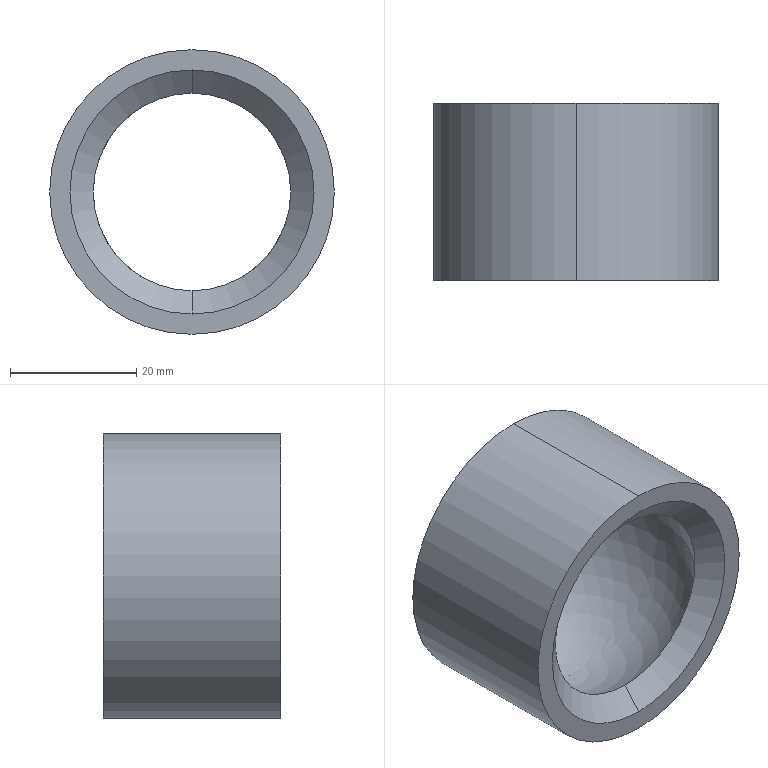Part | SolidWorks | features Revolution 1 | 1 solid | 8 faces | box 45 x 28 x 45 mm | volume 14324 mm3 | cone 2 | sphere 2 | cylinder 2 | plane 2 | commonest cylinder face diameters 45 x2
STEP:
#1=CARTESIAN_POINT('',(-15.612,-12.5,0.));
#2=VERTEX_POINT('',#1);
#3=CARTESIAN_POINT('',(0.,-12.5,15.612));
#4=VERTEX_POINT('',#3);
#5=CARTESIAN_POINT('',(0.,-12.5,0.));
#6=DIRECTION('',(0.,1.,0.));
#7=DIRECTION('',(0.,0.,1.));
#8=AXIS2_PLACEMENT_3D('',#5,#6,#7);
#9=CIRCLE('',#8,15.612);
#10=EDGE_CURVE('',#2,#4,#9,.T.);
#11=ORIENTED_EDGE('',*,*,#10,.T.);
#12=CARTESIAN_POINT('',(0.,-15.5,19.3));
#13=VERTEX_POINT('',#12);
#14=CARTESIAN_POINT('',(0.,-12.5,15.612));
#15=DIRECTION('',(0.,-0.6311,0.7757));
#16=VECTOR('',#15,1000.);
#17=LINE('',#14,#16);
#18=EDGE_CURVE('',#4,#13,#17,.T.);
#19=ORIENTED_EDGE('',*,*,#18,.T.);
#20=CARTESIAN_POINT('',(0.,-15.5,-19.3));
#21=VERTEX_POINT('',#20);
#22=CARTESIAN_POINT('',(0.,-15.5,0.));
#23=DIRECTION('',(0.,1.,0.));
#24=DIRECTION('',(0.,0.,1.));
#25=AXIS2_PLACEMENT_3D('',#22,#23,#24);
#26=CIRCLE('',#25,19.3);
#27=EDGE_CURVE('',#21,#13,#26,.T.);
#28=ORIENTED_EDGE('',*,*,#27,.F.);
#29=CARTESIAN_POINT('',(0.,-12.5,-15.612));
#30=VERTEX_POINT('',#29);
#31=CARTESIAN_POINT('',(0.,-12.5,-15.612));
#32=DIRECTION('',(0.,-0.6311,-0.7757));
#33=VECTOR('',#32,1000.);
#34=LINE('',#31,#33);
#35=EDGE_CURVE('',#30,#21,#34,.T.);
#36=ORIENTED_EDGE('',*,*,#35,.F.);
#37=CARTESIAN_POINT('',(0.,-12.5,0.));
#38=DIRECTION('',(0.,1.,0.));
#39=DIRECTION('',(0.,0.,1.));
#40=AXIS2_PLACEMENT_3D('',#37,#38,#39);
#41=CIRCLE('',#40,15.612);
#42=EDGE_CURVE('',#30,#2,#41,.T.);
#43=ORIENTED_EDGE('',*,*,#42,.T.);
#44=EDGE_LOOP('',(#11,#19,#28,#36,#43));
#45=FACE_OUTER_BOUND('',#44,.T.);
#46=CARTESIAN_POINT('',(0.,-12.5,0.));
#47=DIRECTION('',(0.,-1.,0.));
#48=DIRECTION('',(0.,0.,-1.));
#49=AXIS2_PLACEMENT_3D('',#46,#47,#48);
#50=CONICAL_SURFACE('',#49,15.612,0.8878);
#51=ADVANCED_FACE('',(#45),#50,.F.);
#52=ORIENTED_EDGE('',*,*,#10,.F.);
#53=CARTESIAN_POINT('',(-15.612,12.5,0.));
#54=VERTEX_POINT('',#53);
#55=CARTESIAN_POINT('',(0.,0.,0.));
#56=DIRECTION('',(0.,0.,-1.));
#57=DIRECTION('',(-1.,0.,0.));
#58=AXIS2_PLACEMENT_3D('',#55,#56,#57);
#59=CIRCLE('',#58,20.);
#60=EDGE_CURVE('',#2,#54,#59,.T.);
#61=ORIENTED_EDGE('',*,*,#60,.T.);
#62=CARTESIAN_POINT('',(15.612,12.5,0.));
#63=VERTEX_POINT('',#62);
#64=CARTESIAN_POINT('',(0.,12.5,0.));
#65=DIRECTION('',(0.,1.,0.));
#66=DIRECTION('',(0.,0.,1.));
#67=AXIS2_PLACEMENT_3D('',#64,#65,#66);
#68=CIRCLE('',#67,15.612);
#69=EDGE_CURVE('',#54,#63,#68,.T.);
#70=ORIENTED_EDGE('',*,*,#69,.T.);
#71=CARTESIAN_POINT('',(15.612,-12.5,0.));
#72=VERTEX_POINT('',#71);
#73=CARTESIAN_POINT('',(0.,0.,0.));
#74=DIRECTION('',(0.,0.,1.));
#75=DIRECTION('',(1.,0.,0.));
#76=AXIS2_PLACEMENT_3D('',#73,#74,#75);
#77=CIRCLE('',#76,20.);
#78=EDGE_CURVE('',#72,#63,#77,.T.);
#79=ORIENTED_EDGE('',*,*,#78,.F.);
#80=CARTESIAN_POINT('',(0.,-12.5,0.));
#81=DIRECTION('',(0.,1.,0.));
#82=DIRECTION('',(0.,0.,1.));
#83=AXIS2_PLACEMENT_3D('',#80,#81,#82);
#84=CIRCLE('',#83,15.612);
#85=EDGE_CURVE('',#4,#72,#84,.T.);
#86=ORIENTED_EDGE('',*,*,#85,.F.);
#87=EDGE_LOOP('',(#52,#61,#70,#79,#86));
#88=FACE_OUTER_BOUND('',#87,.T.);
#89=CARTESIAN_POINT('',(0.,0.,0.));
#90=DIRECTION('',(0.,0.,-1.));
#91=DIRECTION('',(1.,0.,0.));
#92=AXIS2_PLACEMENT_3D('',#89,#90,#91);
#93=SPHERICAL_SURFACE('',#92,20.);
#94=ADVANCED_FACE('',(#88),#93,.F.);
#95=CARTESIAN_POINT('',(0.,-15.5,22.5));
#96=VERTEX_POINT('',#95);
#97=CARTESIAN_POINT('',(0.,-15.5,-22.5));
#98=VERTEX_POINT('',#97);
#99=CARTESIAN_POINT('',(0.,-15.5,0.));
#100=DIRECTION('',(0.,1.,0.));
#101=DIRECTION('',(0.,0.,1.));
#102=AXIS2_PLACEMENT_3D('',#99,#100,#101);
#103=CIRCLE('',#102,22.5);
#104=EDGE_CURVE('',#96,#98,#103,.T.);
#105=ORIENTED_EDGE('',*,*,#104,.T.);
#106=CARTESIAN_POINT('',(0.,12.5,-22.5));
#107=VERTEX_POINT('',#106);
#108=CARTESIAN_POINT('',(0.,29.923,-22.5));
#109=DIRECTION('',(0.,1.,0.));
#110=VECTOR('',#109,1000.);
#111=LINE('',#108,#110);
#112=EDGE_CURVE('',#98,#107,#111,.T.);
#113=ORIENTED_EDGE('',*,*,#112,.T.);
#114=CARTESIAN_POINT('',(0.,12.5,22.5));
#115=VERTEX_POINT('',#114);
#116=CARTESIAN_POINT('',(0.,12.5,0.));
#117=DIRECTION('',(0.,1.,0.));
#118=DIRECTION('',(0.,0.,1.));
#119=AXIS2_PLACEMENT_3D('',#116,#117,#118);
#120=CIRCLE('',#119,22.5);
#121=EDGE_CURVE('',#115,#107,#120,.T.);
#122=ORIENTED_EDGE('',*,*,#121,.F.);
#123=CARTESIAN_POINT('',(0.,29.923,22.5));
#124=DIRECTION('',(0.,1.,0.));
#125=VECTOR('',#124,1000.);
#126=LINE('',#123,#125);
#127=EDGE_CURVE('',#96,#115,#126,.T.);
#128=ORIENTED_EDGE('',*,*,#127,.F.);
#129=EDGE_LOOP('',(#105,#113,#122,#128));
#130=FACE_OUTER_BOUND('',#129,.T.);
#131=CARTESIAN_POINT('',(0.,29.923,0.));
#132=DIRECTION('',(0.,1.,0.));
#133=DIRECTION('',(0.,0.,1.));
#134=AXIS2_PLACEMENT_3D('',#131,#132,#133);
#135=CYLINDRICAL_SURFACE('',#134,22.5);
#136=ADVANCED_FACE('',(#130),#135,.T.);
#137=ORIENTED_EDGE('',*,*,#112,.F.);
#138=CARTESIAN_POINT('',(0.,-15.5,0.));
#139=DIRECTION('',(0.,1.,0.));
#140=DIRECTION('',(0.,0.,1.));
#141=AXIS2_PLACEMENT_3D('',#138,#139,#140);
#142=CIRCLE('',#141,22.5);
#143=EDGE_CURVE('',#98,#96,#142,.T.);
#144=ORIENTED_EDGE('',*,*,#143,.T.);
#145=ORIENTED_EDGE('',*,*,#127,.T.);
#146=CARTESIAN_POINT('',(0.,12.5,0.));
#147=DIRECTION('',(0.,1.,0.));
#148=DIRECTION('',(0.,0.,1.));
#149=AXIS2_PLACEMENT_3D('',#146,#147,#148);
#150=CIRCLE('',#149,22.5);
#151=EDGE_CURVE('',#107,#115,#150,.T.);
#152=ORIENTED_EDGE('',*,*,#151,.F.);
#153=EDGE_LOOP('',(#137,#144,#145,#152));
#154=FACE_OUTER_BOUND('',#153,.T.);
#155=CARTESIAN_POINT('',(0.,29.923,0.));
#156=DIRECTION('',(0.,1.,0.));
#157=DIRECTION('',(0.,0.,1.));
#158=AXIS2_PLACEMENT_3D('',#155,#156,#157);
#159=CYLINDRICAL_SURFACE('',#158,22.5);
#160=ADVANCED_FACE('',(#154),#159,.T.);
#161=CARTESIAN_POINT('',(0.,12.5,0.));
#162=DIRECTION('',(0.,1.,0.));
#163=DIRECTION('',(0.,0.,1.));
#164=AXIS2_PLACEMENT_3D('',#161,#162,#163);
#165=CIRCLE('',#164,15.612);
#166=EDGE_CURVE('',#63,#54,#165,.T.);
#167=ORIENTED_EDGE('',*,*,#166,.F.);
#168=ORIENTED_EDGE('',*,*,#69,.F.);
#169=EDGE_LOOP('',(#167,#168));
#170=FACE_BOUND('',#169,.T.);
#171=ORIENTED_EDGE('',*,*,#121,.T.);
#172=ORIENTED_EDGE('',*,*,#151,.T.);
#173=EDGE_LOOP('',(#171,#172));
#174=FACE_OUTER_BOUND('',#173,.T.);
#175=CARTESIAN_POINT('',(15.612,12.5,0.));
#176=DIRECTION('',(0.,-1.,0.));
#177=DIRECTION('',(0.,0.,-1.));
#178=AXIS2_PLACEMENT_3D('',#175,#176,#177);
#179=PLANE('',#178);
#180=ADVANCED_FACE('',(#170,#174),#179,.F.);
#181=ORIENTED_EDGE('',*,*,#60,.F.);
#182=ORIENTED_EDGE('',*,*,#42,.F.);
#183=CARTESIAN_POINT('',(0.,-12.5,0.));
#184=DIRECTION('',(0.,1.,0.));
#185=DIRECTION('',(0.,0.,1.));
#186=AXIS2_PLACEMENT_3D('',#183,#184,#185);
#187=CIRCLE('',#186,15.612);
#188=EDGE_CURVE('',#72,#30,#187,.T.);
#189=ORIENTED_EDGE('',*,*,#188,.F.);
#190=ORIENTED_EDGE('',*,*,#78,.T.);
#191=ORIENTED_EDGE('',*,*,#166,.T.);
#192=EDGE_LOOP('',(#181,#182,#189,#190,#191));
#193=FACE_OUTER_BOUND('',#192,.T.);
#194=CARTESIAN_POINT('',(0.,0.,0.));
#195=DIRECTION('',(0.,0.,-1.));
#196=DIRECTION('',(1.,0.,0.));
#197=AXIS2_PLACEMENT_3D('',#194,#195,#196);
#198=SPHERICAL_SURFACE('',#197,20.);
#199=ADVANCED_FACE('',(#193),#198,.F.);
#200=ORIENTED_EDGE('',*,*,#18,.F.);
#201=ORIENTED_EDGE('',*,*,#85,.T.);
#202=ORIENTED_EDGE('',*,*,#188,.T.);
#203=ORIENTED_EDGE('',*,*,#35,.T.);
#204=CARTESIAN_POINT('',(0.,-15.5,0.));
#205=DIRECTION('',(0.,1.,0.));
#206=DIRECTION('',(0.,0.,1.));
#207=AXIS2_PLACEMENT_3D('',#204,#205,#206);
#208=CIRCLE('',#207,19.3);
#209=EDGE_CURVE('',#13,#21,#208,.T.);
#210=ORIENTED_EDGE('',*,*,#209,.F.);
#211=EDGE_LOOP('',(#200,#201,#202,#203,#210));
#212=FACE_OUTER_BOUND('',#211,.T.);
#213=CARTESIAN_POINT('',(0.,-12.5,0.));
#214=DIRECTION('',(0.,-1.,0.));
#215=DIRECTION('',(0.,0.,-1.));
#216=AXIS2_PLACEMENT_3D('',#213,#214,#215);
#217=CONICAL_SURFACE('',#216,15.612,0.8878);
#218=ADVANCED_FACE('',(#212),#217,.F.);
#219=ORIENTED_EDGE('',*,*,#104,.F.);
#220=ORIENTED_EDGE('',*,*,#143,.F.);
#221=EDGE_LOOP('',(#219,#220));
#222=FACE_OUTER_BOUND('',#221,.T.);
#223=ORIENTED_EDGE('',*,*,#27,.T.);
#224=ORIENTED_EDGE('',*,*,#209,.T.);
#225=EDGE_LOOP('',(#223,#224));
#226=FACE_BOUND('',#225,.T.);
#227=CARTESIAN_POINT('',(22.5,-15.5,0.));
#228=DIRECTION('',(0.,1.,0.));
#229=DIRECTION('',(0.,0.,1.));
#230=AXIS2_PLACEMENT_3D('',#227,#228,#229);
#231=PLANE('',#230);
#232=ADVANCED_FACE('',(#222,#226),#231,.F.);
#233=CLOSED_SHELL('',(#51,#94,#136,#160,#180,#199,#218,#232));
#234=MANIFOLD_SOLID_BREP('',#233);
#235=CARTESIAN_POINT('',(0.,0.,0.));
#236=DIRECTION('',(0.,0.,1.));
#237=DIRECTION('',(1.,0.,0.));
#238=AXIS2_PLACEMENT_3D('',#235,#236,#237);
#239=(LENGTH_UNIT()NAMED_UNIT(*)SI_UNIT(.MILLI.,.METRE.));
#240=UNCERTAINTY_MEASURE_WITH_UNIT(LENGTH_MEASURE(0.00001),#239,'','');
#241=(NAMED_UNIT(*)PLANE_ANGLE_UNIT()SI_UNIT($,.RADIAN.));
#242=(NAMED_UNIT(*)SI_UNIT($,.STERADIAN.)SOLID_ANGLE_UNIT());
#243=(GEOMETRIC_REPRESENTATION_CONTEXT(3)GLOBAL_UNCERTAINTY_ASSIGNED_CONTEXT((#240))GLOBAL_UNIT_ASSIGNED_CONTEXT((#239,#241,#242))REPRESENTATION_CONTEXT('',''));
#244=ADVANCED_BREP_SHAPE_REPRESENTATION('',(#234,#238),#243);